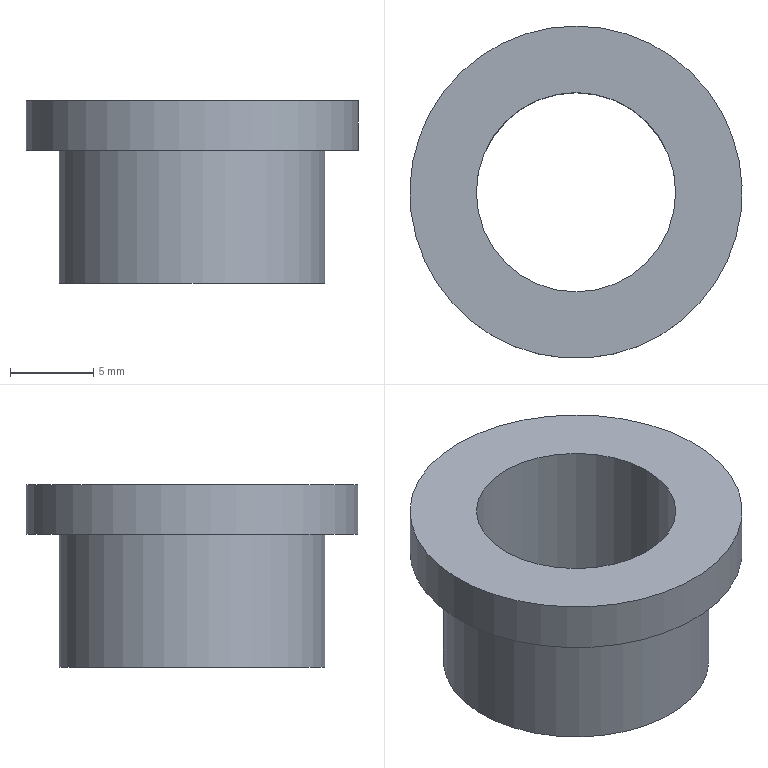Part | STEP file | 1-58B | 1 solid | 6 faces | box 20 x 20 x 11 mm | volume 1307 mm3 | plane 3 | cylinder 3 | commonest cylinder face diameters 12 x1 16 x1 20 x1
STEP:
#1=CARTESIAN_POINT('',(0.,0.,0.));
#2=DIRECTION('',(0.,0.,1.));
#3=DIRECTION('',(1.,0.,0.));
#4=AXIS2_PLACEMENT_3D('',#1,#2,#3);
#5=CARTESIAN_POINT('',(0.,8.,-8.));
#6=VERTEX_POINT('',#5);
#7=CARTESIAN_POINT('',(0.,0.,-8.));
#8=DIRECTION('',(0.,0.,1.));
#9=DIRECTION('',(0.,1.,0.));
#10=AXIS2_PLACEMENT_3D('',#7,#8,#9);
#11=CIRCLE('',#10,8.);
#12=CARTESIAN_POINT('',(0.,-2.144,-8.));
#13=DIRECTION('',(0.,0.,1.));
#14=DIRECTION('',(1.,0.,0.));
#15=AXIS2_PLACEMENT_3D('',#12,#13,#14);
#16=PLANE('',#15);
#17=CARTESIAN_POINT('',(0.,2.144));
#18=DIRECTION('',(0.,1.));
#19=AXIS2_PLACEMENT_2D('',#17,#18);
#20=CIRCLE('',#19,8.);
#21=(GEOMETRIC_REPRESENTATION_CONTEXT(2)PARAMETRIC_REPRESENTATION_CONTEXT()REPRESENTATION_CONTEXT('',''));
#22=DEFINITIONAL_REPRESENTATION('',(#20),#21);
#23=PCURVE('',#16,#22);
#24=CARTESIAN_POINT('',(0.,0.,0.));
#25=DIRECTION('',(0.,0.,-1.));
#26=DIRECTION('',(0.,1.,0.));
#27=AXIS2_PLACEMENT_3D('',#24,#25,#26);
#28=CYLINDRICAL_SURFACE('',#27,8.);
#29=CARTESIAN_POINT('',(6.283,8.));
#30=DIRECTION('',(-1.,0.));
#31=VECTOR('',#30,1.);
#32=LINE('',#29,#31);
#33=(GEOMETRIC_REPRESENTATION_CONTEXT(2)PARAMETRIC_REPRESENTATION_CONTEXT()REPRESENTATION_CONTEXT('',''));
#34=DEFINITIONAL_REPRESENTATION('',(#32),#33);
#35=PCURVE('',#28,#34);
#36=SURFACE_CURVE('',#11,(#23,#35),.PCURVE_S1.);
#37=EDGE_CURVE('',#6,#6,#36,.T.);
#38=ORIENTED_EDGE('',*,*,#37,.T.);
#39=EDGE_LOOP('',(#38));
#40=FACE_BOUND('',#39,.F.);
#41=CARTESIAN_POINT('',(0.,6.,-8.));
#42=VERTEX_POINT('',#41);
#43=CARTESIAN_POINT('',(0.,0.,-8.));
#44=DIRECTION('',(0.,0.,-1.));
#45=DIRECTION('',(0.,1.,0.));
#46=AXIS2_PLACEMENT_3D('',#43,#44,#45);
#47=CIRCLE('',#46,6.);
#48=CARTESIAN_POINT('',(0.,8.144));
#49=CARTESIAN_POINT('',(10.392,8.144));
#50=CARTESIAN_POINT('',(5.196,-0.8564));
#51=CARTESIAN_POINT('',(0.,-9.856));
#52=CARTESIAN_POINT('',(-5.196,-0.8564));
#53=CARTESIAN_POINT('',(-10.392,8.144));
#54=CARTESIAN_POINT('',(0.,8.144));
#55=(BOUNDED_CURVE()B_SPLINE_CURVE(2,(#48,#49,#50,#51,#52,#53,#54),.UNSPECIFIED.,.T.,.F.)B_SPLINE_CURVE_WITH_KNOTS((1,2,2,2,2,1),(-2.094,0.,2.094,4.189,6.283,8.378),.UNSPECIFIED.)CURVE()GEOMETRIC_REPRESENTATION_ITEM()RATIONAL_B_SPLINE_CURVE((1.,0.5,1.,0.5,1.,0.5,1.))REPRESENTATION_ITEM(''));
#56=(GEOMETRIC_REPRESENTATION_CONTEXT(2)PARAMETRIC_REPRESENTATION_CONTEXT()REPRESENTATION_CONTEXT('',''));
#57=DEFINITIONAL_REPRESENTATION('',(#55),#56);
#58=PCURVE('',#16,#57);
#59=CARTESIAN_POINT('',(0.,0.,3.));
#60=DIRECTION('',(0.,0.,-1.));
#61=DIRECTION('',(0.,1.,0.));
#62=AXIS2_PLACEMENT_3D('',#59,#60,#61);
#63=CYLINDRICAL_SURFACE('',#62,6.);
#64=CARTESIAN_POINT('',(0.,11.));
#65=DIRECTION('',(1.,0.));
#66=VECTOR('',#65,1.);
#67=LINE('',#64,#66);
#68=(GEOMETRIC_REPRESENTATION_CONTEXT(2)PARAMETRIC_REPRESENTATION_CONTEXT()REPRESENTATION_CONTEXT('',''));
#69=DEFINITIONAL_REPRESENTATION('',(#67),#68);
#70=PCURVE('',#63,#69);
#71=SURFACE_CURVE('',#47,(#58,#70),.PCURVE_S1.);
#72=EDGE_CURVE('',#42,#42,#71,.T.);
#73=ORIENTED_EDGE('',*,*,#72,.T.);
#74=EDGE_LOOP('',(#73));
#75=FACE_BOUND('',#74,.F.);
#76=ADVANCED_FACE('',(#40,#75),#16,.F.);
#77=CARTESIAN_POINT('',(0.,8.,0.));
#78=VERTEX_POINT('',#77);
#79=CARTESIAN_POINT('',(0.,8.,0.));
#80=DIRECTION('',(0.,0.,-1.));
#81=VECTOR('',#80,1.);
#82=LINE('',#79,#81);
#83=CARTESIAN_POINT('',(6.283,0.));
#84=DIRECTION('',(0.,1.));
#85=VECTOR('',#84,1.);
#86=LINE('',#83,#85);
#87=(GEOMETRIC_REPRESENTATION_CONTEXT(2)PARAMETRIC_REPRESENTATION_CONTEXT()REPRESENTATION_CONTEXT('',''));
#88=DEFINITIONAL_REPRESENTATION('',(#86),#87);
#89=PCURVE('',#28,#88);
#90=CARTESIAN_POINT('',(0.,0.));
#91=DIRECTION('',(0.,1.));
#92=VECTOR('',#91,1.);
#93=LINE('',#90,#92);
#94=(GEOMETRIC_REPRESENTATION_CONTEXT(2)PARAMETRIC_REPRESENTATION_CONTEXT()REPRESENTATION_CONTEXT('',''));
#95=DEFINITIONAL_REPRESENTATION('',(#93),#94);
#96=PCURVE('',#28,#95);
#97=SEAM_CURVE('',#82,(#89,#96),.PCURVE_S1.);
#98=EDGE_CURVE('',#78,#6,#97,.T.);
#99=ORIENTED_EDGE('',*,*,#98,.T.);
#100=ORIENTED_EDGE('',*,*,#37,.T.);
#101=ORIENTED_EDGE('',*,*,#98,.F.);
#102=CARTESIAN_POINT('',(0.,0.,0.));
#103=DIRECTION('',(0.,0.,1.));
#104=DIRECTION('',(0.,1.,0.));
#105=AXIS2_PLACEMENT_3D('',#102,#103,#104);
#106=CIRCLE('',#105,8.);
#107=CARTESIAN_POINT('',(6.283,0.));
#108=DIRECTION('',(-1.,0.));
#109=VECTOR('',#108,1.);
#110=LINE('',#107,#109);
#111=(GEOMETRIC_REPRESENTATION_CONTEXT(2)PARAMETRIC_REPRESENTATION_CONTEXT()REPRESENTATION_CONTEXT('',''));
#112=DEFINITIONAL_REPRESENTATION('',(#110),#111);
#113=PCURVE('',#28,#112);
#114=CARTESIAN_POINT('',(0.,-2.679,0.));
#115=DIRECTION('',(0.,0.,1.));
#116=DIRECTION('',(1.,0.,0.));
#117=AXIS2_PLACEMENT_3D('',#114,#115,#116);
#118=PLANE('',#117);
#119=CARTESIAN_POINT('',(0.,2.679));
#120=DIRECTION('',(0.,1.));
#121=AXIS2_PLACEMENT_2D('',#119,#120);
#122=CIRCLE('',#121,8.);
#123=(GEOMETRIC_REPRESENTATION_CONTEXT(2)PARAMETRIC_REPRESENTATION_CONTEXT()REPRESENTATION_CONTEXT('',''));
#124=DEFINITIONAL_REPRESENTATION('',(#122),#123);
#125=PCURVE('',#118,#124);
#126=SURFACE_CURVE('',#106,(#113,#125),.PCURVE_S1.);
#127=EDGE_CURVE('',#78,#78,#126,.T.);
#128=ORIENTED_EDGE('',*,*,#127,.F.);
#129=EDGE_LOOP('',(#99,#100,#101,#128));
#130=FACE_BOUND('',#129,.T.);
#131=ADVANCED_FACE('',(#130),#28,.T.);
#132=ORIENTED_EDGE('',*,*,#72,.F.);
#133=CARTESIAN_POINT('',(0.,6.,3.));
#134=VERTEX_POINT('',#133);
#135=CARTESIAN_POINT('',(0.,6.,-8.));
#136=DIRECTION('',(0.,0.,1.));
#137=VECTOR('',#136,1.);
#138=LINE('',#135,#137);
#139=CARTESIAN_POINT('',(0.,11.));
#140=DIRECTION('',(0.,-1.));
#141=VECTOR('',#140,1.);
#142=LINE('',#139,#141);
#143=(GEOMETRIC_REPRESENTATION_CONTEXT(2)PARAMETRIC_REPRESENTATION_CONTEXT()REPRESENTATION_CONTEXT('',''));
#144=DEFINITIONAL_REPRESENTATION('',(#142),#143);
#145=PCURVE('',#63,#144);
#146=CARTESIAN_POINT('',(6.283,11.));
#147=DIRECTION('',(0.,-1.));
#148=VECTOR('',#147,1.);
#149=LINE('',#146,#148);
#150=(GEOMETRIC_REPRESENTATION_CONTEXT(2)PARAMETRIC_REPRESENTATION_CONTEXT()REPRESENTATION_CONTEXT('',''));
#151=DEFINITIONAL_REPRESENTATION('',(#149),#150);
#152=PCURVE('',#63,#151);
#153=SEAM_CURVE('',#138,(#145,#152),.PCURVE_S1.);
#154=EDGE_CURVE('',#42,#134,#153,.T.);
#155=ORIENTED_EDGE('',*,*,#154,.T.);
#156=CARTESIAN_POINT('',(0.,0.,3.));
#157=DIRECTION('',(0.,0.,-1.));
#158=DIRECTION('',(0.,1.,0.));
#159=AXIS2_PLACEMENT_3D('',#156,#157,#158);
#160=CIRCLE('',#159,6.);
#161=CARTESIAN_POINT('',(0.,0.));
#162=DIRECTION('',(1.,0.));
#163=VECTOR('',#162,1.);
#164=LINE('',#161,#163);
#165=(GEOMETRIC_REPRESENTATION_CONTEXT(2)PARAMETRIC_REPRESENTATION_CONTEXT()REPRESENTATION_CONTEXT('',''));
#166=DEFINITIONAL_REPRESENTATION('',(#164),#165);
#167=PCURVE('',#63,#166);
#168=CARTESIAN_POINT('',(0.,-2.679,3.));
#169=DIRECTION('',(0.,0.,1.));
#170=DIRECTION('',(1.,0.,0.));
#171=AXIS2_PLACEMENT_3D('',#168,#169,#170);
#172=PLANE('',#171);
#173=CARTESIAN_POINT('',(0.,8.679));
#174=CARTESIAN_POINT('',(10.392,8.679));
#175=CARTESIAN_POINT('',(5.196,-0.3205));
#176=CARTESIAN_POINT('',(0.,-9.321));
#177=CARTESIAN_POINT('',(-5.196,-0.3205));
#178=CARTESIAN_POINT('',(-10.392,8.679));
#179=CARTESIAN_POINT('',(0.,8.679));
#180=(BOUNDED_CURVE()B_SPLINE_CURVE(2,(#173,#174,#175,#176,#177,#178,#179),.UNSPECIFIED.,.T.,.F.)B_SPLINE_CURVE_WITH_KNOTS((1,2,2,2,2,1),(-2.094,0.,2.094,4.189,6.283,8.378),.UNSPECIFIED.)CURVE()GEOMETRIC_REPRESENTATION_ITEM()RATIONAL_B_SPLINE_CURVE((1.,0.5,1.,0.5,1.,0.5,1.))REPRESENTATION_ITEM(''));
#181=(GEOMETRIC_REPRESENTATION_CONTEXT(2)PARAMETRIC_REPRESENTATION_CONTEXT()REPRESENTATION_CONTEXT('',''));
#182=DEFINITIONAL_REPRESENTATION('',(#180),#181);
#183=PCURVE('',#172,#182);
#184=SURFACE_CURVE('',#160,(#167,#183),.PCURVE_S1.);
#185=EDGE_CURVE('',#134,#134,#184,.T.);
#186=ORIENTED_EDGE('',*,*,#185,.T.);
#187=ORIENTED_EDGE('',*,*,#154,.F.);
#188=EDGE_LOOP('',(#132,#155,#186,#187));
#189=FACE_BOUND('',#188,.F.);
#190=ADVANCED_FACE('',(#189),#63,.F.);
#191=CARTESIAN_POINT('',(0.,10.,0.));
#192=VERTEX_POINT('',#191);
#193=CARTESIAN_POINT('',(0.,0.,0.));
#194=DIRECTION('',(0.,0.,1.));
#195=DIRECTION('',(0.,1.,0.));
#196=AXIS2_PLACEMENT_3D('',#193,#194,#195);
#197=CIRCLE('',#196,10.);
#198=CARTESIAN_POINT('',(0.,2.679));
#199=DIRECTION('',(0.,1.));
#200=AXIS2_PLACEMENT_2D('',#198,#199);
#201=CIRCLE('',#200,10.);
#202=(GEOMETRIC_REPRESENTATION_CONTEXT(2)PARAMETRIC_REPRESENTATION_CONTEXT()REPRESENTATION_CONTEXT('',''));
#203=DEFINITIONAL_REPRESENTATION('',(#201),#202);
#204=PCURVE('',#118,#203);
#205=CARTESIAN_POINT('',(0.,0.,0.));
#206=DIRECTION('',(0.,0.,1.));
#207=DIRECTION('',(0.,1.,0.));
#208=AXIS2_PLACEMENT_3D('',#205,#206,#207);
#209=CYLINDRICAL_SURFACE('',#208,10.);
#210=CARTESIAN_POINT('',(0.,0.));
#211=DIRECTION('',(1.,0.));
#212=VECTOR('',#211,1.);
#213=LINE('',#210,#212);
#214=(GEOMETRIC_REPRESENTATION_CONTEXT(2)PARAMETRIC_REPRESENTATION_CONTEXT()REPRESENTATION_CONTEXT('',''));
#215=DEFINITIONAL_REPRESENTATION('',(#213),#214);
#216=PCURVE('',#209,#215);
#217=SURFACE_CURVE('',#197,(#204,#216),.PCURVE_S1.);
#218=EDGE_CURVE('',#192,#192,#217,.T.);
#219=ORIENTED_EDGE('',*,*,#218,.T.);
#220=EDGE_LOOP('',(#219));
#221=FACE_BOUND('',#220,.F.);
#222=ORIENTED_EDGE('',*,*,#127,.F.);
#223=EDGE_LOOP('',(#222));
#224=FACE_BOUND('',#223,.F.);
#225=ADVANCED_FACE('',(#221,#224),#118,.F.);
#226=ORIENTED_EDGE('',*,*,#218,.T.);
#227=CARTESIAN_POINT('',(0.,10.,3.));
#228=VERTEX_POINT('',#227);
#229=CARTESIAN_POINT('',(0.,10.,0.));
#230=DIRECTION('',(0.,0.,1.));
#231=VECTOR('',#230,1.);
#232=LINE('',#229,#231);
#233=CARTESIAN_POINT('',(6.283,0.));
#234=DIRECTION('',(0.,1.));
#235=VECTOR('',#234,1.);
#236=LINE('',#233,#235);
#237=(GEOMETRIC_REPRESENTATION_CONTEXT(2)PARAMETRIC_REPRESENTATION_CONTEXT()REPRESENTATION_CONTEXT('',''));
#238=DEFINITIONAL_REPRESENTATION('',(#236),#237);
#239=PCURVE('',#209,#238);
#240=CARTESIAN_POINT('',(0.,0.));
#241=DIRECTION('',(0.,1.));
#242=VECTOR('',#241,1.);
#243=LINE('',#240,#242);
#244=(GEOMETRIC_REPRESENTATION_CONTEXT(2)PARAMETRIC_REPRESENTATION_CONTEXT()REPRESENTATION_CONTEXT('',''));
#245=DEFINITIONAL_REPRESENTATION('',(#243),#244);
#246=PCURVE('',#209,#245);
#247=SEAM_CURVE('',#232,(#239,#246),.PCURVE_S1.);
#248=EDGE_CURVE('',#192,#228,#247,.T.);
#249=ORIENTED_EDGE('',*,*,#248,.T.);
#250=CARTESIAN_POINT('',(0.,0.,3.));
#251=DIRECTION('',(0.,0.,1.));
#252=DIRECTION('',(0.,1.,0.));
#253=AXIS2_PLACEMENT_3D('',#250,#251,#252);
#254=CIRCLE('',#253,10.);
#255=CARTESIAN_POINT('',(0.,3.));
#256=DIRECTION('',(1.,0.));
#257=VECTOR('',#256,1.);
#258=LINE('',#255,#257);
#259=(GEOMETRIC_REPRESENTATION_CONTEXT(2)PARAMETRIC_REPRESENTATION_CONTEXT()REPRESENTATION_CONTEXT('',''));
#260=DEFINITIONAL_REPRESENTATION('',(#258),#259);
#261=PCURVE('',#209,#260);
#262=CARTESIAN_POINT('',(0.,2.679));
#263=DIRECTION('',(0.,1.));
#264=AXIS2_PLACEMENT_2D('',#262,#263);
#265=CIRCLE('',#264,10.);
#266=(GEOMETRIC_REPRESENTATION_CONTEXT(2)PARAMETRIC_REPRESENTATION_CONTEXT()REPRESENTATION_CONTEXT('',''));
#267=DEFINITIONAL_REPRESENTATION('',(#265),#266);
#268=PCURVE('',#172,#267);
#269=SURFACE_CURVE('',#254,(#261,#268),.PCURVE_S1.);
#270=EDGE_CURVE('',#228,#228,#269,.T.);
#271=ORIENTED_EDGE('',*,*,#270,.F.);
#272=ORIENTED_EDGE('',*,*,#248,.F.);
#273=EDGE_LOOP('',(#226,#249,#271,#272));
#274=FACE_BOUND('',#273,.T.);
#275=ADVANCED_FACE('',(#274),#209,.T.);
#276=ORIENTED_EDGE('',*,*,#270,.T.);
#277=EDGE_LOOP('',(#276));
#278=FACE_BOUND('',#277,.T.);
#279=ORIENTED_EDGE('',*,*,#185,.T.);
#280=EDGE_LOOP('',(#279));
#281=FACE_BOUND('',#280,.T.);
#282=ADVANCED_FACE('',(#278,#281),#172,.T.);
#283=CLOSED_SHELL('',(#76,#131,#190,#225,#275,#282));
#284=MANIFOLD_SOLID_BREP('',#283);
#285=(LENGTH_UNIT()NAMED_UNIT(*)SI_UNIT(.MILLI.,.METRE.));
#286=UNCERTAINTY_MEASURE_WITH_UNIT(LENGTH_MEASURE(0.0000001),#285,'','');
#287=(NAMED_UNIT(*)PLANE_ANGLE_UNIT()SI_UNIT($,.RADIAN.));
#288=(NAMED_UNIT(*)SI_UNIT($,.STERADIAN.)SOLID_ANGLE_UNIT());
#289=(GEOMETRIC_REPRESENTATION_CONTEXT(3)GLOBAL_UNCERTAINTY_ASSIGNED_CONTEXT((#286))GLOBAL_UNIT_ASSIGNED_CONTEXT((#285,#287,#288))REPRESENTATION_CONTEXT('',''));
#290=ADVANCED_BREP_SHAPE_REPRESENTATION('',(#4,#284),#289);